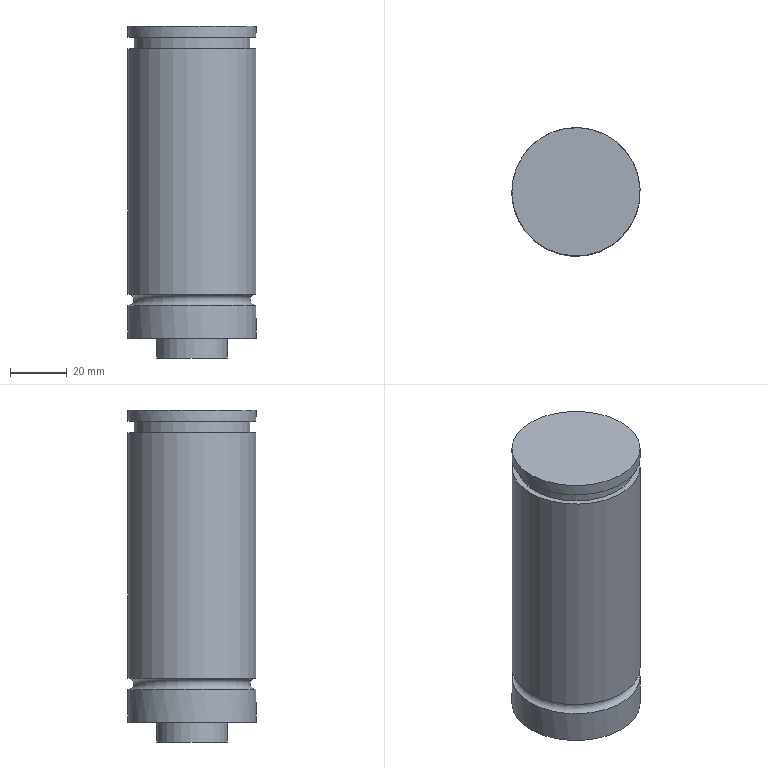Part | NX | features MAIN_BODY 2 | 1 solid | 11 faces | box 45.2 x 45.2 x 117 mm | volume 177998 mm3 | cylinder 5 | plane 5 | torus 1 | commonest cylinder face diameters 45.2 x3 25 x1 41.2 x1
STEP:
#1=CARTESIAN_POINT('',(1554.516,-169.516,377.));
#2=VERTEX_POINT('',#1);
#3=CARTESIAN_POINT('',(1538.536,-153.536,377.));
#4=DIRECTION('',(0.,0.,1.));
#5=DIRECTION('',(0.7071,-0.7071,0.));
#6=AXIS2_PLACEMENT_3D('',#3,#4,#5);
#7=CIRCLE('',#6,22.6);
#8=EDGE_CURVE('',#2,#2,#7,.F.);
#9=ORIENTED_EDGE('',*,*,#8,.T.);
#10=EDGE_LOOP('',(#9));
#11=FACE_BOUND('',#10,.T.);
#12=CARTESIAN_POINT('',(1554.516,-169.516,290.5));
#13=VERTEX_POINT('',#12);
#14=CARTESIAN_POINT('',(1538.536,-153.536,290.5));
#15=DIRECTION('',(0.,0.,1.));
#16=DIRECTION('',(0.7071,-0.7071,0.));
#17=AXIS2_PLACEMENT_3D('',#14,#15,#16);
#18=CIRCLE('',#17,22.6);
#19=EDGE_CURVE('',#13,#13,#18,.T.);
#20=ORIENTED_EDGE('',*,*,#19,.T.);
#21=EDGE_LOOP('',(#20));
#22=FACE_BOUND('',#21,.T.);
#23=CARTESIAN_POINT('',(1538.536,-153.536,275.));
#24=DIRECTION('',(0.,0.,1.));
#25=DIRECTION('',(0.7071,-0.7071,0.));
#26=AXIS2_PLACEMENT_3D('',#23,#24,#25);
#27=CYLINDRICAL_SURFACE('',#26,22.6);
#28=ADVANCED_FACE('',(#11,#22),#27,.T.);
#29=CARTESIAN_POINT('',(1522.555,-137.555,275.));
#30=VERTEX_POINT('',#29);
#31=CARTESIAN_POINT('',(1538.536,-153.536,275.));
#32=DIRECTION('',(0.,0.,-1.));
#33=DIRECTION('',(-0.7071,0.7071,0.));
#34=AXIS2_PLACEMENT_3D('',#31,#32,#33);
#35=CIRCLE('',#34,22.6);
#36=EDGE_CURVE('',#30,#30,#35,.T.);
#37=ORIENTED_EDGE('',*,*,#36,.T.);
#38=EDGE_LOOP('',(#37));
#39=FACE_BOUND('',#38,.T.);
#40=CARTESIAN_POINT('',(1529.697,-144.697,275.));
#41=VERTEX_POINT('',#40);
#42=CARTESIAN_POINT('',(1538.536,-153.536,275.));
#43=DIRECTION('',(0.,0.,-1.));
#44=DIRECTION('',(-0.7071,0.7071,0.));
#45=AXIS2_PLACEMENT_3D('',#42,#43,#44);
#46=CIRCLE('',#45,12.5);
#47=EDGE_CURVE('',#41,#41,#46,.T.);
#48=ORIENTED_EDGE('',*,*,#47,.F.);
#49=EDGE_LOOP('',(#48));
#50=FACE_BOUND('',#49,.T.);
#51=CARTESIAN_POINT('',(1538.536,-153.536,275.));
#52=DIRECTION('',(0.,0.,-1.));
#53=DIRECTION('',(-0.7071,0.7071,0.));
#54=AXIS2_PLACEMENT_3D('',#51,#52,#53);
#55=PLANE('',#54);
#56=ADVANCED_FACE('',(#39,#50),#55,.T.);
#57=CARTESIAN_POINT('',(1554.516,-169.516,286.5));
#58=VERTEX_POINT('',#57);
#59=CARTESIAN_POINT('',(1538.536,-153.536,286.5));
#60=DIRECTION('',(0.,0.,1.));
#61=DIRECTION('',(0.7071,-0.7071,0.));
#62=AXIS2_PLACEMENT_3D('',#59,#60,#61);
#63=CIRCLE('',#62,22.6);
#64=EDGE_CURVE('',#58,#58,#63,.F.);
#65=ORIENTED_EDGE('',*,*,#64,.T.);
#66=EDGE_LOOP('',(#65));
#67=FACE_BOUND('',#66,.T.);
#68=ORIENTED_EDGE('',*,*,#36,.F.);
#69=EDGE_LOOP('',(#68));
#70=FACE_BOUND('',#69,.T.);
#71=CARTESIAN_POINT('',(1538.536,-153.536,275.));
#72=DIRECTION('',(0.,0.,1.));
#73=DIRECTION('',(0.7071,-0.7071,0.));
#74=AXIS2_PLACEMENT_3D('',#71,#72,#73);
#75=CYLINDRICAL_SURFACE('',#74,22.6);
#76=ADVANCED_FACE('',(#67,#70),#75,.T.);
#77=ORIENTED_EDGE('',*,*,#47,.T.);
#78=EDGE_LOOP('',(#77));
#79=FACE_BOUND('',#78,.T.);
#80=CARTESIAN_POINT('',(1529.697,-144.697,268.));
#81=VERTEX_POINT('',#80);
#82=CARTESIAN_POINT('',(1538.536,-153.536,268.));
#83=DIRECTION('',(0.,0.,-1.));
#84=DIRECTION('',(-0.7071,0.7071,0.));
#85=AXIS2_PLACEMENT_3D('',#82,#83,#84);
#86=CIRCLE('',#85,12.5);
#87=EDGE_CURVE('',#81,#81,#86,.T.);
#88=ORIENTED_EDGE('',*,*,#87,.F.);
#89=EDGE_LOOP('',(#88));
#90=FACE_BOUND('',#89,.T.);
#91=CARTESIAN_POINT('',(1538.536,-153.536,273.));
#92=DIRECTION('',(0.,0.,1.));
#93=DIRECTION('',(0.7071,-0.7071,0.));
#94=AXIS2_PLACEMENT_3D('',#91,#92,#93);
#95=CYLINDRICAL_SURFACE('',#94,12.5);
#96=ADVANCED_FACE('',(#79,#90),#95,.T.);
#97=ORIENTED_EDGE('',*,*,#64,.F.);
#98=EDGE_LOOP('',(#97));
#99=FACE_BOUND('',#98,.T.);
#100=ORIENTED_EDGE('',*,*,#19,.F.);
#101=EDGE_LOOP('',(#100));
#102=FACE_BOUND('',#101,.T.);
#103=CARTESIAN_POINT('',(1538.536,-153.536,288.5));
#104=DIRECTION('',(0.,0.,1.));
#105=DIRECTION('',(0.7071,-0.7071,0.));
#106=AXIS2_PLACEMENT_3D('',#103,#104,#105);
#107=TOROIDAL_SURFACE('',#106,22.6,2.);
#108=ADVANCED_FACE('',(#99,#102),#107,.F.);
#109=CARTESIAN_POINT('',(1523.969,-138.969,377.));
#110=VERTEX_POINT('',#109);
#111=CARTESIAN_POINT('',(1538.536,-153.536,377.));
#112=DIRECTION('',(0.,0.,-1.));
#113=DIRECTION('',(-0.7071,0.7071,0.));
#114=AXIS2_PLACEMENT_3D('',#111,#112,#113);
#115=CIRCLE('',#114,20.6);
#116=EDGE_CURVE('',#110,#110,#115,.T.);
#117=ORIENTED_EDGE('',*,*,#116,.T.);
#118=EDGE_LOOP('',(#117));
#119=FACE_BOUND('',#118,.T.);
#120=ORIENTED_EDGE('',*,*,#8,.F.);
#121=EDGE_LOOP('',(#120));
#122=FACE_BOUND('',#121,.T.);
#123=CARTESIAN_POINT('',(1538.536,-153.536,377.));
#124=DIRECTION('',(0.,0.,1.));
#125=DIRECTION('',(0.7071,-0.7071,0.));
#126=AXIS2_PLACEMENT_3D('',#123,#124,#125);
#127=PLANE('',#126);
#128=ADVANCED_FACE('',(#119,#122),#127,.T.);
#129=CARTESIAN_POINT('',(1523.969,-138.969,381.));
#130=VERTEX_POINT('',#129);
#131=CARTESIAN_POINT('',(1538.536,-153.536,381.));
#132=DIRECTION('',(0.,0.,-1.));
#133=DIRECTION('',(-0.7071,0.7071,0.));
#134=AXIS2_PLACEMENT_3D('',#131,#132,#133);
#135=CIRCLE('',#134,20.6);
#136=EDGE_CURVE('',#130,#130,#135,.T.);
#137=ORIENTED_EDGE('',*,*,#136,.F.);
#138=EDGE_LOOP('',(#137));
#139=FACE_BOUND('',#138,.T.);
#140=CARTESIAN_POINT('',(1554.516,-169.516,381.));
#141=VERTEX_POINT('',#140);
#142=CARTESIAN_POINT('',(1538.536,-153.536,381.));
#143=DIRECTION('',(0.,0.,1.));
#144=DIRECTION('',(0.7071,-0.7071,0.));
#145=AXIS2_PLACEMENT_3D('',#142,#143,#144);
#146=CIRCLE('',#145,22.6);
#147=EDGE_CURVE('',#141,#141,#146,.T.);
#148=ORIENTED_EDGE('',*,*,#147,.F.);
#149=EDGE_LOOP('',(#148));
#150=FACE_BOUND('',#149,.T.);
#151=CARTESIAN_POINT('',(1538.536,-153.536,381.));
#152=DIRECTION('',(0.,0.,1.));
#153=DIRECTION('',(0.7071,-0.7071,0.));
#154=AXIS2_PLACEMENT_3D('',#151,#152,#153);
#155=PLANE('',#154);
#156=ADVANCED_FACE('',(#139,#150),#155,.F.);
#157=ORIENTED_EDGE('',*,*,#116,.F.);
#158=EDGE_LOOP('',(#157));
#159=FACE_BOUND('',#158,.T.);
#160=ORIENTED_EDGE('',*,*,#136,.T.);
#161=EDGE_LOOP('',(#160));
#162=FACE_BOUND('',#161,.T.);
#163=CARTESIAN_POINT('',(1538.536,-153.536,381.));
#164=DIRECTION('',(0.,0.,-1.));
#165=DIRECTION('',(-0.7071,0.7071,0.));
#166=AXIS2_PLACEMENT_3D('',#163,#164,#165);
#167=CYLINDRICAL_SURFACE('',#166,20.6);
#168=ADVANCED_FACE('',(#159,#162),#167,.T.);
#169=CARTESIAN_POINT('',(1522.555,-137.555,385.));
#170=VERTEX_POINT('',#169);
#171=CARTESIAN_POINT('',(1538.536,-153.536,385.));
#172=DIRECTION('',(0.,0.,-1.));
#173=DIRECTION('',(-0.7071,0.7071,0.));
#174=AXIS2_PLACEMENT_3D('',#171,#172,#173);
#175=CIRCLE('',#174,22.6);
#176=EDGE_CURVE('',#170,#170,#175,.T.);
#177=ORIENTED_EDGE('',*,*,#176,.F.);
#178=EDGE_LOOP('',(#177));
#179=FACE_BOUND('',#178,.T.);
#180=CARTESIAN_POINT('',(1538.536,-153.536,385.));
#181=DIRECTION('',(0.,0.,-1.));
#182=DIRECTION('',(-0.7071,0.7071,0.));
#183=AXIS2_PLACEMENT_3D('',#180,#181,#182);
#184=PLANE('',#183);
#185=ADVANCED_FACE('',(#179),#184,.F.);
#186=ORIENTED_EDGE('',*,*,#147,.T.);
#187=EDGE_LOOP('',(#186));
#188=FACE_BOUND('',#187,.T.);
#189=ORIENTED_EDGE('',*,*,#176,.T.);
#190=EDGE_LOOP('',(#189));
#191=FACE_BOUND('',#190,.T.);
#192=CARTESIAN_POINT('',(1538.536,-153.536,275.));
#193=DIRECTION('',(0.,0.,1.));
#194=DIRECTION('',(0.7071,-0.7071,0.));
#195=AXIS2_PLACEMENT_3D('',#192,#193,#194);
#196=CYLINDRICAL_SURFACE('',#195,22.6);
#197=ADVANCED_FACE('',(#188,#191),#196,.T.);
#198=ORIENTED_EDGE('',*,*,#87,.T.);
#199=EDGE_LOOP('',(#198));
#200=FACE_BOUND('',#199,.T.);
#201=CARTESIAN_POINT('',(1538.536,-153.536,268.));
#202=DIRECTION('',(0.,0.,-1.));
#203=DIRECTION('',(-0.7071,0.7071,0.));
#204=AXIS2_PLACEMENT_3D('',#201,#202,#203);
#205=PLANE('',#204);
#206=ADVANCED_FACE('',(#200),#205,.T.);
#207=CLOSED_SHELL('',(#28,#56,#76,#96,#108,#128,#156,#168,#185,#197,#206));
#208=MANIFOLD_SOLID_BREP('',#207);
#209=(LENGTH_UNIT()NAMED_UNIT(*)SI_UNIT(.MILLI.,.METRE.));
#210=UNCERTAINTY_MEASURE_WITH_UNIT(LENGTH_MEASURE(0.00001),#209,'','');
#211=(NAMED_UNIT(*)PLANE_ANGLE_UNIT()SI_UNIT($,.RADIAN.));
#212=(NAMED_UNIT(*)SI_UNIT($,.STERADIAN.)SOLID_ANGLE_UNIT());
#213=(GEOMETRIC_REPRESENTATION_CONTEXT(3)GLOBAL_UNCERTAINTY_ASSIGNED_CONTEXT((#210))GLOBAL_UNIT_ASSIGNED_CONTEXT((#209,#211,#212))REPRESENTATION_CONTEXT('',''));
#214=ADVANCED_BREP_SHAPE_REPRESENTATION('',(#208),#213);